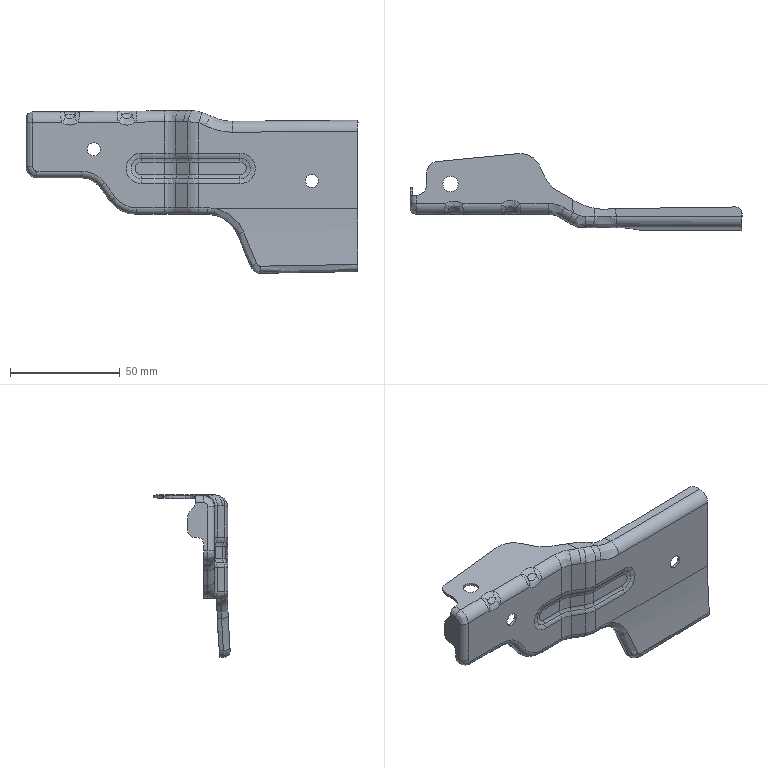Part | 1 solid | 234 faces | box 151.475 x 34.925 x 74.203 mm | volume 12104 mm3 | cylinder 91 | spline 84 | plane 41 | torus 11 | other 7 | commonest cylinder face diameters 10 x15 6 x13 7.6 x13 3.6 x7 8 x7 20 x7